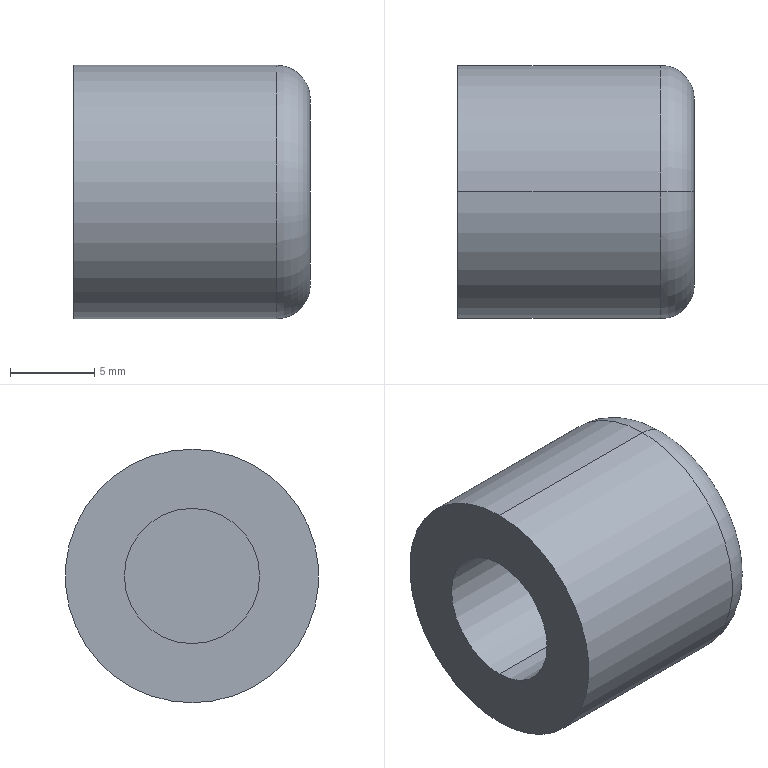Part | SolidWorks | features Revolution 1 | 1 solid | 9 faces | box 14 x 15 x 15 mm | volume 1834 mm3 | cylinder 4 | plane 3 | torus 2 | commonest cylinder face diameters 8 x2 15 x2
STEP:
#1=CARTESIAN_POINT('',(-0.5512,0.,0.1575));
#2=VERTEX_POINT('',#1);
#3=CARTESIAN_POINT('',(-0.5512,0.,-0.1575));
#4=VERTEX_POINT('',#3);
#5=CARTESIAN_POINT('',(-0.5512,0.,0.));
#6=DIRECTION('',(1.,0.,0.));
#7=DIRECTION('',(0.,0.,-1.));
#8=AXIS2_PLACEMENT_3D('',#5,#6,#7);
#9=CIRCLE('',#8,0.1575);
#10=EDGE_CURVE('',#2,#4,#9,.T.);
#11=ORIENTED_EDGE('',*,*,#10,.F.);
#12=CARTESIAN_POINT('',(-0.07941,0.,0.1575));
#13=VERTEX_POINT('',#12);
#14=CARTESIAN_POINT('',(0.,0.,0.1575));
#15=DIRECTION('',(1.,0.,0.));
#16=VECTOR('',#15,39.37);
#17=LINE('',#14,#16);
#18=EDGE_CURVE('',#2,#13,#17,.T.);
#19=ORIENTED_EDGE('',*,*,#18,.T.);
#20=CARTESIAN_POINT('',(-0.07941,0.,-0.1575));
#21=VERTEX_POINT('',#20);
#22=CARTESIAN_POINT('',(-0.07941,0.,0.));
#23=DIRECTION('',(1.,0.,0.));
#24=DIRECTION('',(0.,0.,-1.));
#25=AXIS2_PLACEMENT_3D('',#22,#23,#24);
#26=CIRCLE('',#25,0.1575);
#27=EDGE_CURVE('',#13,#21,#26,.T.);
#28=ORIENTED_EDGE('',*,*,#27,.T.);
#29=CARTESIAN_POINT('',(0.,0.,-0.1575));
#30=DIRECTION('',(1.,0.,0.));
#31=VECTOR('',#30,39.37);
#32=LINE('',#29,#31);
#33=EDGE_CURVE('',#4,#21,#32,.T.);
#34=ORIENTED_EDGE('',*,*,#33,.F.);
#35=EDGE_LOOP('',(#11,#19,#28,#34));
#36=FACE_OUTER_BOUND('',#35,.T.);
#37=CARTESIAN_POINT('',(0.,0.,0.));
#38=DIRECTION('',(1.,0.,0.));
#39=DIRECTION('',(0.,0.,-1.));
#40=AXIS2_PLACEMENT_3D('',#37,#38,#39);
#41=CYLINDRICAL_SURFACE('',#40,0.1575);
#42=ADVANCED_FACE('',(#36),#41,.F.);
#43=CARTESIAN_POINT('',(-0.5512,0.,-0.2953));
#44=VERTEX_POINT('',#43);
#45=CARTESIAN_POINT('',(-0.5512,0.,0.2953));
#46=VERTEX_POINT('',#45);
#47=CARTESIAN_POINT('',(-0.5512,0.,0.));
#48=DIRECTION('',(1.,0.,0.));
#49=DIRECTION('',(0.,0.,-1.));
#50=AXIS2_PLACEMENT_3D('',#47,#48,#49);
#51=CIRCLE('',#50,0.2953);
#52=EDGE_CURVE('',#44,#46,#51,.T.);
#53=ORIENTED_EDGE('',*,*,#52,.T.);
#54=CARTESIAN_POINT('',(-0.07874,0.,0.2953));
#55=VERTEX_POINT('',#54);
#56=CARTESIAN_POINT('',(0.,0.,0.2953));
#57=DIRECTION('',(1.,0.,0.));
#58=VECTOR('',#57,39.37);
#59=LINE('',#56,#58);
#60=EDGE_CURVE('',#46,#55,#59,.T.);
#61=ORIENTED_EDGE('',*,*,#60,.T.);
#62=CARTESIAN_POINT('',(-0.07874,0.,-0.2953));
#63=VERTEX_POINT('',#62);
#64=CARTESIAN_POINT('',(-0.07874,0.,0.));
#65=DIRECTION('',(1.,0.,0.));
#66=DIRECTION('',(0.,0.,-1.));
#67=AXIS2_PLACEMENT_3D('',#64,#65,#66);
#68=CIRCLE('',#67,0.2953);
#69=EDGE_CURVE('',#63,#55,#68,.T.);
#70=ORIENTED_EDGE('',*,*,#69,.F.);
#71=CARTESIAN_POINT('',(0.,0.,-0.2953));
#72=DIRECTION('',(1.,0.,0.));
#73=VECTOR('',#72,39.37);
#74=LINE('',#71,#73);
#75=EDGE_CURVE('',#44,#63,#74,.T.);
#76=ORIENTED_EDGE('',*,*,#75,.F.);
#77=EDGE_LOOP('',(#53,#61,#70,#76));
#78=FACE_OUTER_BOUND('',#77,.T.);
#79=CARTESIAN_POINT('',(0.,0.,0.));
#80=DIRECTION('',(1.,0.,0.));
#81=DIRECTION('',(0.,0.,-1.));
#82=AXIS2_PLACEMENT_3D('',#79,#80,#81);
#83=CYLINDRICAL_SURFACE('',#82,0.2953);
#84=ADVANCED_FACE('',(#78),#83,.T.);
#85=ORIENTED_EDGE('',*,*,#69,.T.);
#86=CARTESIAN_POINT('',(0.,0.,0.2165));
#87=VERTEX_POINT('',#86);
#88=CARTESIAN_POINT('',(-0.07874,0.,0.2165));
#89=DIRECTION('',(0.,1.,0.));
#90=DIRECTION('',(0.,0.,1.));
#91=AXIS2_PLACEMENT_3D('',#88,#89,#90);
#92=CIRCLE('',#91,0.07874);
#93=EDGE_CURVE('',#55,#87,#92,.T.);
#94=ORIENTED_EDGE('',*,*,#93,.T.);
#95=CARTESIAN_POINT('',(0.,0.,-0.2165));
#96=VERTEX_POINT('',#95);
#97=CARTESIAN_POINT('',(0.,0.,0.));
#98=DIRECTION('',(1.,0.,0.));
#99=DIRECTION('',(0.,0.,-1.));
#100=AXIS2_PLACEMENT_3D('',#97,#98,#99);
#101=CIRCLE('',#100,0.2165);
#102=EDGE_CURVE('',#96,#87,#101,.T.);
#103=ORIENTED_EDGE('',*,*,#102,.F.);
#104=CARTESIAN_POINT('',(-0.07874,0.,-0.2165));
#105=DIRECTION('',(0.,-1.,0.));
#106=DIRECTION('',(0.,0.,-1.));
#107=AXIS2_PLACEMENT_3D('',#104,#105,#106);
#108=CIRCLE('',#107,0.07874);
#109=EDGE_CURVE('',#63,#96,#108,.T.);
#110=ORIENTED_EDGE('',*,*,#109,.F.);
#111=EDGE_LOOP('',(#85,#94,#103,#110));
#112=FACE_OUTER_BOUND('',#111,.T.);
#113=CARTESIAN_POINT('',(-0.07874,0.,0.));
#114=DIRECTION('',(1.,0.,0.));
#115=DIRECTION('',(0.,0.,-1.));
#116=AXIS2_PLACEMENT_3D('',#113,#114,#115);
#117=TOROIDAL_SURFACE('',#116,0.2165,0.07874);
#118=ADVANCED_FACE('',(#112),#117,.T.);
#119=ORIENTED_EDGE('',*,*,#102,.T.);
#120=CARTESIAN_POINT('',(0.,0.,0.));
#121=DIRECTION('',(1.,0.,0.));
#122=DIRECTION('',(0.,0.,-1.));
#123=AXIS2_PLACEMENT_3D('',#120,#121,#122);
#124=CIRCLE('',#123,0.2165);
#125=EDGE_CURVE('',#87,#96,#124,.T.);
#126=ORIENTED_EDGE('',*,*,#125,.T.);
#127=EDGE_LOOP('',(#119,#126));
#128=FACE_OUTER_BOUND('',#127,.T.);
#129=CARTESIAN_POINT('',(0.,0.,0.));
#130=DIRECTION('',(1.,0.,0.));
#131=DIRECTION('',(0.,0.,-1.));
#132=AXIS2_PLACEMENT_3D('',#129,#130,#131);
#133=PLANE('',#132);
#134=ADVANCED_FACE('',(#128),#133,.T.);
#135=ORIENTED_EDGE('',*,*,#93,.F.);
#136=CARTESIAN_POINT('',(-0.07874,0.,0.));
#137=DIRECTION('',(1.,0.,0.));
#138=DIRECTION('',(0.,0.,-1.));
#139=AXIS2_PLACEMENT_3D('',#136,#137,#138);
#140=CIRCLE('',#139,0.2953);
#141=EDGE_CURVE('',#55,#63,#140,.T.);
#142=ORIENTED_EDGE('',*,*,#141,.T.);
#143=ORIENTED_EDGE('',*,*,#109,.T.);
#144=ORIENTED_EDGE('',*,*,#125,.F.);
#145=EDGE_LOOP('',(#135,#142,#143,#144));
#146=FACE_OUTER_BOUND('',#145,.T.);
#147=CARTESIAN_POINT('',(-0.07874,0.,0.));
#148=DIRECTION('',(1.,0.,0.));
#149=DIRECTION('',(0.,0.,-1.));
#150=AXIS2_PLACEMENT_3D('',#147,#148,#149);
#151=TOROIDAL_SURFACE('',#150,0.2165,0.07874);
#152=ADVANCED_FACE('',(#146),#151,.T.);
#153=ORIENTED_EDGE('',*,*,#60,.F.);
#154=CARTESIAN_POINT('',(-0.5512,0.,0.));
#155=DIRECTION('',(1.,0.,0.));
#156=DIRECTION('',(0.,0.,-1.));
#157=AXIS2_PLACEMENT_3D('',#154,#155,#156);
#158=CIRCLE('',#157,0.2953);
#159=EDGE_CURVE('',#46,#44,#158,.T.);
#160=ORIENTED_EDGE('',*,*,#159,.T.);
#161=ORIENTED_EDGE('',*,*,#75,.T.);
#162=ORIENTED_EDGE('',*,*,#141,.F.);
#163=EDGE_LOOP('',(#153,#160,#161,#162));
#164=FACE_OUTER_BOUND('',#163,.T.);
#165=CARTESIAN_POINT('',(0.,0.,0.));
#166=DIRECTION('',(1.,0.,0.));
#167=DIRECTION('',(0.,0.,-1.));
#168=AXIS2_PLACEMENT_3D('',#165,#166,#167);
#169=CYLINDRICAL_SURFACE('',#168,0.2953);
#170=ADVANCED_FACE('',(#164),#169,.T.);
#171=CARTESIAN_POINT('',(-0.5512,0.,0.));
#172=DIRECTION('',(1.,0.,0.));
#173=DIRECTION('',(0.,0.,-1.));
#174=AXIS2_PLACEMENT_3D('',#171,#172,#173);
#175=CIRCLE('',#174,0.1575);
#176=EDGE_CURVE('',#4,#2,#175,.T.);
#177=ORIENTED_EDGE('',*,*,#176,.T.);
#178=ORIENTED_EDGE('',*,*,#10,.T.);
#179=EDGE_LOOP('',(#177,#178));
#180=FACE_BOUND('',#179,.T.);
#181=ORIENTED_EDGE('',*,*,#52,.F.);
#182=ORIENTED_EDGE('',*,*,#159,.F.);
#183=EDGE_LOOP('',(#181,#182));
#184=FACE_OUTER_BOUND('',#183,.T.);
#185=CARTESIAN_POINT('',(-0.5512,0.2953,0.));
#186=DIRECTION('',(-1.,0.,0.));
#187=DIRECTION('',(0.,0.,1.));
#188=AXIS2_PLACEMENT_3D('',#185,#186,#187);
#189=PLANE('',#188);
#190=ADVANCED_FACE('',(#180,#184),#189,.T.);
#191=ORIENTED_EDGE('',*,*,#18,.F.);
#192=ORIENTED_EDGE('',*,*,#176,.F.);
#193=ORIENTED_EDGE('',*,*,#33,.T.);
#194=CARTESIAN_POINT('',(-0.07941,0.,0.));
#195=DIRECTION('',(1.,0.,0.));
#196=DIRECTION('',(0.,0.,-1.));
#197=AXIS2_PLACEMENT_3D('',#194,#195,#196);
#198=CIRCLE('',#197,0.1575);
#199=EDGE_CURVE('',#21,#13,#198,.T.);
#200=ORIENTED_EDGE('',*,*,#199,.T.);
#201=EDGE_LOOP('',(#191,#192,#193,#200));
#202=FACE_OUTER_BOUND('',#201,.T.);
#203=CARTESIAN_POINT('',(0.,0.,0.));
#204=DIRECTION('',(1.,0.,0.));
#205=DIRECTION('',(0.,0.,-1.));
#206=AXIS2_PLACEMENT_3D('',#203,#204,#205);
#207=CYLINDRICAL_SURFACE('',#206,0.1575);
#208=ADVANCED_FACE('',(#202),#207,.F.);
#209=ORIENTED_EDGE('',*,*,#199,.F.);
#210=ORIENTED_EDGE('',*,*,#27,.F.);
#211=EDGE_LOOP('',(#209,#210));
#212=FACE_OUTER_BOUND('',#211,.T.);
#213=CARTESIAN_POINT('',(-0.07941,0.1575,0.));
#214=DIRECTION('',(-1.,0.,0.));
#215=DIRECTION('',(0.,0.,1.));
#216=AXIS2_PLACEMENT_3D('',#213,#214,#215);
#217=PLANE('',#216);
#218=ADVANCED_FACE('',(#212),#217,.T.);
#219=CLOSED_SHELL('',(#42,#84,#118,#134,#152,#170,#190,#208,#218));
#220=MANIFOLD_SOLID_BREP('',#219);
#221=CARTESIAN_POINT('',(0.,0.,0.));
#222=DIRECTION('',(0.,0.,1.));
#223=DIRECTION('',(1.,0.,0.));
#224=AXIS2_PLACEMENT_3D('',#221,#222,#223);
#225=(LENGTH_UNIT()NAMED_UNIT(*)SI_UNIT($,.METRE.));
#226=LENGTH_MEASURE_WITH_UNIT(LENGTH_MEASURE(0.0254),#225);
#227=DIMENSIONAL_EXPONENTS(1.,0.,0.,0.,0.,0.,0.);
#228=(CONVERSION_BASED_UNIT('INCH',#226)LENGTH_UNIT()NAMED_UNIT(#227));
#229=UNCERTAINTY_MEASURE_WITH_UNIT(LENGTH_MEASURE(0.00001),#228,'','');
#230=(NAMED_UNIT(*)PLANE_ANGLE_UNIT()SI_UNIT($,.RADIAN.));
#231=(NAMED_UNIT(*)SI_UNIT($,.STERADIAN.)SOLID_ANGLE_UNIT());
#232=(GEOMETRIC_REPRESENTATION_CONTEXT(3)GLOBAL_UNCERTAINTY_ASSIGNED_CONTEXT((#229))GLOBAL_UNIT_ASSIGNED_CONTEXT((#228,#230,#231))REPRESENTATION_CONTEXT('',''));
#233=ADVANCED_BREP_SHAPE_REPRESENTATION('',(#220,#224),#232);